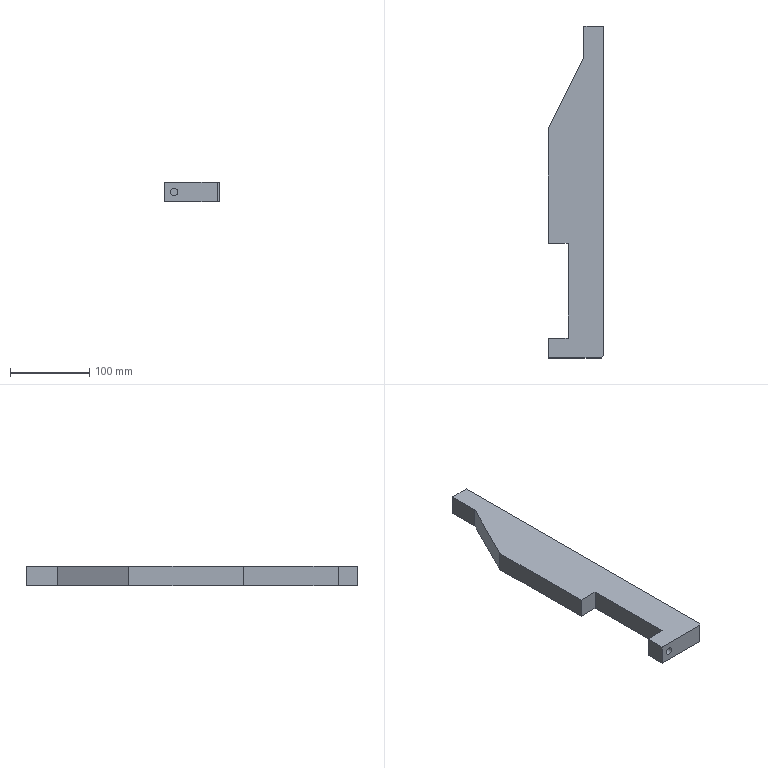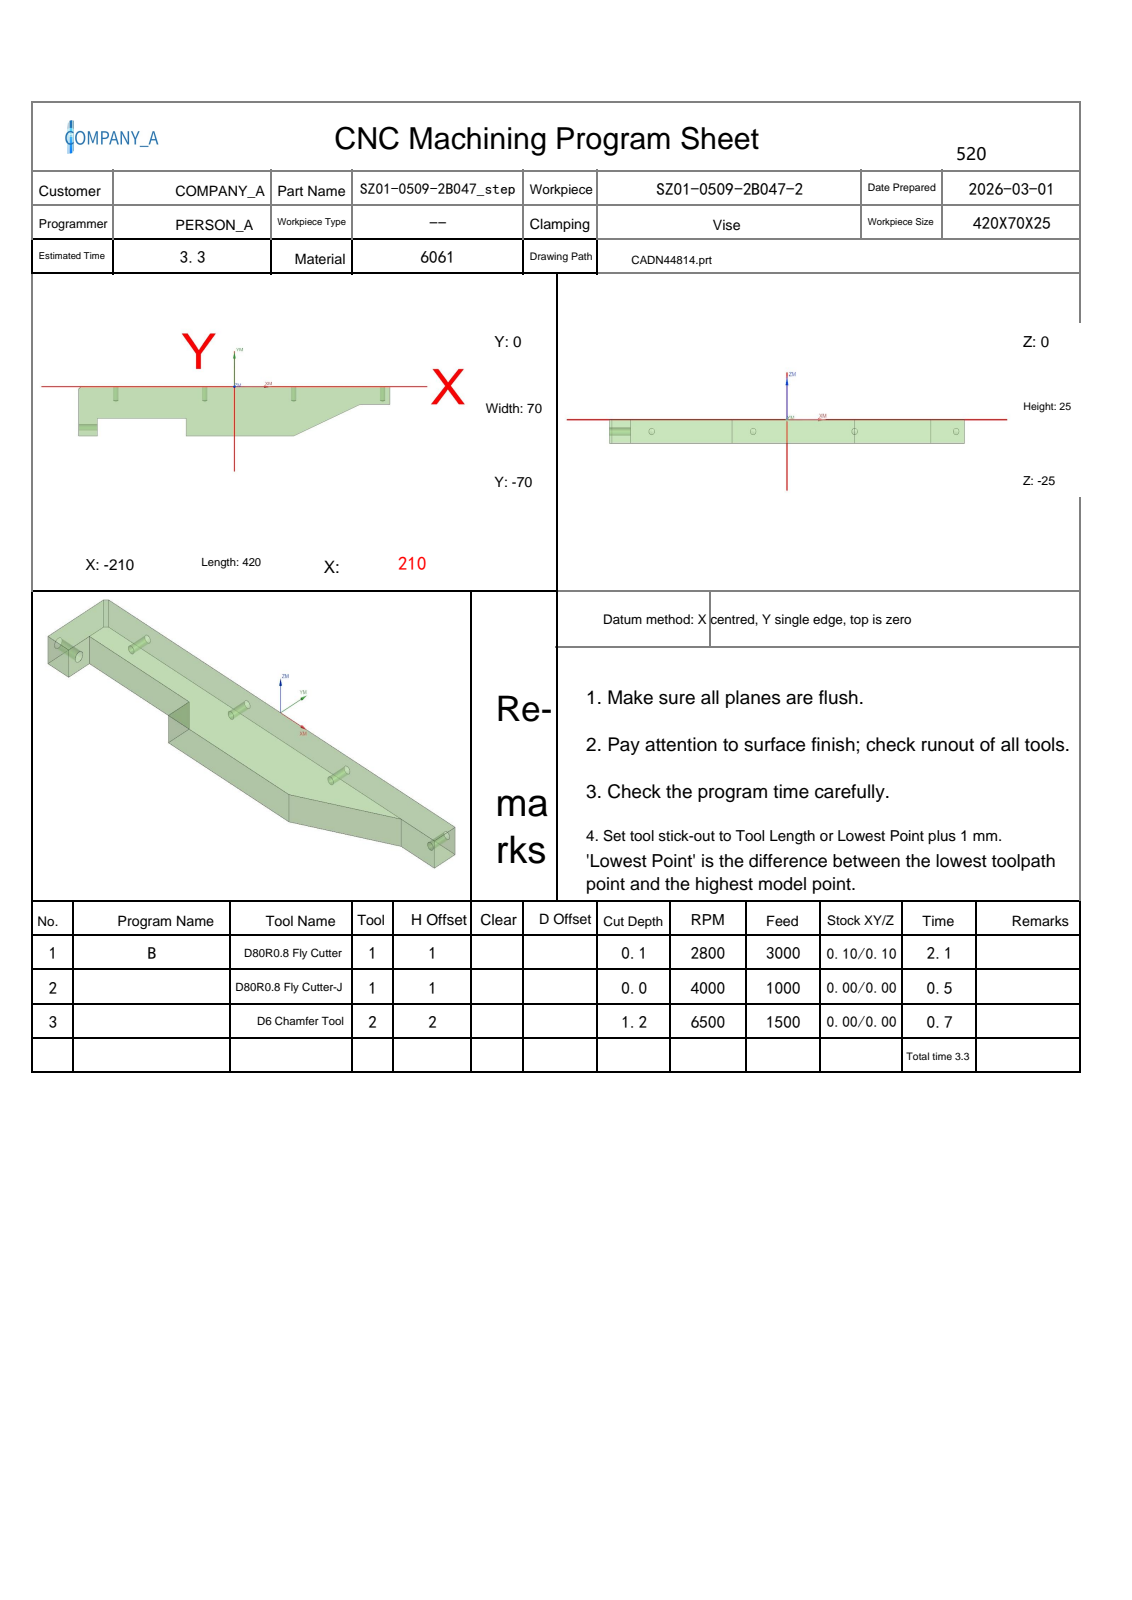NC program | NX | posted by the shop | part box 70 x 420 x 25 mm
Whole program:
%
O0001
(Machine time: 3.78 MIN)
(===Total Tool:2===)
(T1=D80R0.8 fly cutter D=80.  R=0.8  D-  H01 Z=0.    )
(T2=D6 chamfer tool   D=6.   R=0.   D-  H02 Z=-1.2  )
G80 G90 G17 G49 G40
G91 G28 Z0
M01
N1 T01 M06
(D80R0.8 fly cutter  D=80. R=0.8 H=01 ce=0.10 di=0.10)
G00 G90 G54 X-262.097 Y-35. M03 S2800
G43 H01 Z50.
M08
Z6.011
G01 Z4.011 F3000.
X-250.097
X250.097
X262.097
Z6.011
G00 X-262.097
Z5.522
G01 Z3.522
X-250.097
X250.097
X262.097
Z5.522
G00 X-262.097
Z5.033
G01 Z3.033
X-250.097
X250.097
X262.097
Z5.033
G00 X-262.097
Z4.544
G01 Z2.544
X-250.097
X250.097
X262.097
Z4.544
G00 Z50.
X-262.097
Z4.056
G01 Z2.056
X-250.097
X250.097
X262.097
Z4.056
G00 Z50.
X-262.097
Z3.567
G01 Z1.567
X-250.097
X250.097
X262.097
Z3.567
G00 Z50.
X-262.097
Z3.078
G01 Z1.078
X-250.097
X250.097
X262.097
Z3.078
G00 Z50.
X-262.097
Z2.589
G01 Z.589
X-250.097
X250.097
X262.097
Z2.589
G00 Z50.
X-262.097
Z2.1
G01 Z.1
X-250.097
X250.097
X262.097
Z2.1
G00 Z50.
G91 G28 Z0.0
M05
M09
G91 G28 Z0.0
M01
N2 T01 M06
(D80R0.8 fly cutter-J  D=80. R=0.8 H=01 ce=0.00 di=0.00)
G00 G90 G54 X-261.999 Y-35. M03 S4000
G43 H01 Z50.
M08
Z2.
G01 Z0.0 F1000.
X-249.999
X249.999
X261.999
Z2.
G00 Z50.
G91 G28 Z0.0
M05
M09
G91 G28 Z0.0
M01
N3 T02 M06
(D6 chamfer tool  D=6. R=0. H=02 ce=0.00 di=0.00)
G00 G90 G54 X1.114 Y1.227 M03 S6500
G43 H02 Z50.
M08
Z.172
G01 Z-1.2 F1500.
G03 X1.4 Y1.027 I1.286 J1.532
G01 X1.446 Y.997
X1.5 Y1.
X210.
G02 X211. Y0.0 I0.0 J-1.
G01 Y-25.
G02 X210. Y-26. I-1. J0.0
G01 X170.236
X80.447 Y-70.894
X80.23 Y-70.973
X80. Y-71.
X-65.
G02 X-66. Y-70. I0.0 J1.
G01 Y-46.
X-184.
Y-70.
G02 X-185. Y-71. I-1. J0.0
G01 X-210.
G02 X-211. Y-70. I0.0 J1.
G01 Y-3.
X-210.966 Y-2.741
X-210.866 Y-2.5
X-210.707 Y-2.293
X-207.707 Y.707
X-207.5 Y.866
X-207.259 Y.966
X-207. Y1.
X1.5
X1.554 Y.997
X1.6 Y1.027
G03 X1.886 Y1.227 I-1. J1.732
G01 Z.172
G00 Z50.
M05
M09
G91 G28 Z0.0
G91 G28 Y0.0
M30
%